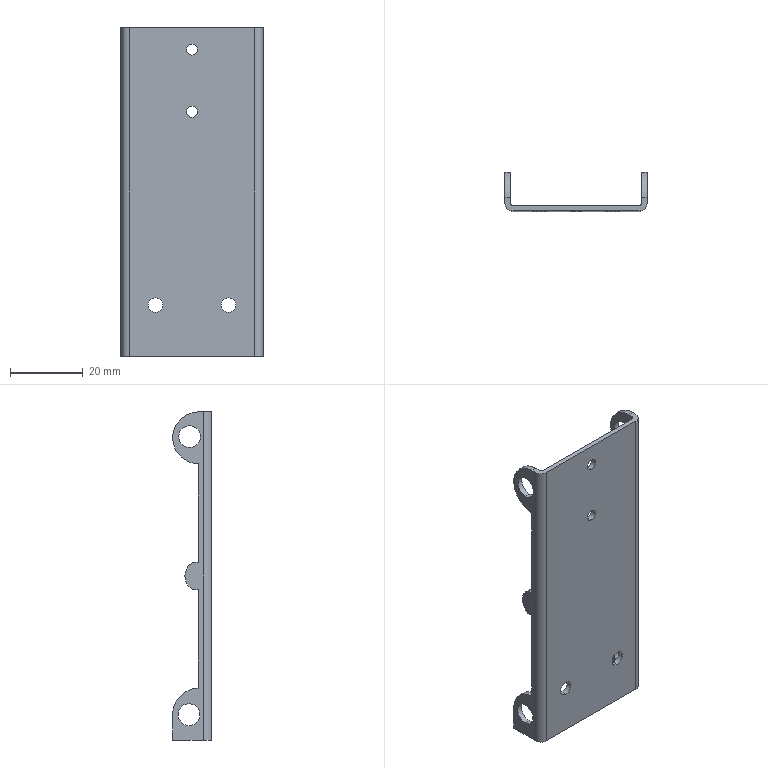Part | SolidWorks | features HoleWzd 4, Fillet 2, ICE 2, Extrusion 1 | 1 solid | 46 faces | box 39 x 10.638 x 90 mm | volume 6007 mm3 | cylinder 28 | plane 18 | commonest cylinder face diameters 6 x8 3 x4 4 x4 9.055 x4 1.473 x2 4.473 x2
STEP:
#1=CARTESIAN_POINT('',(-9.5,-1.5,-7.5));
#2=VERTEX_POINT('',#1);
#3=CARTESIAN_POINT('',(-9.5,-1.5,-4.5));
#4=VERTEX_POINT('',#3);
#5=CARTESIAN_POINT('',(-9.5,-1.5,-6.));
#6=DIRECTION('',(0.,1.,0.));
#7=DIRECTION('',(0.,0.,1.));
#8=AXIS2_PLACEMENT_3D('',#5,#6,#7);
#9=CIRCLE('',#8,1.5);
#10=EDGE_CURVE('',#2,#4,#9,.T.);
#11=ORIENTED_EDGE('',*,*,#10,.F.);
#12=CARTESIAN_POINT('',(-9.5,0.,-7.5));
#13=VERTEX_POINT('',#12);
#14=CARTESIAN_POINT('',(-9.5,0.,-7.5));
#15=DIRECTION('',(0.,1.,0.));
#16=VECTOR('',#15,1000.);
#17=LINE('',#14,#16);
#18=EDGE_CURVE('',#2,#13,#17,.T.);
#19=ORIENTED_EDGE('',*,*,#18,.T.);
#20=CARTESIAN_POINT('',(-9.5,0.,-4.5));
#21=VERTEX_POINT('',#20);
#22=CARTESIAN_POINT('',(-9.5,0.,-6.));
#23=DIRECTION('',(0.,1.,0.));
#24=DIRECTION('',(0.,0.,1.));
#25=AXIS2_PLACEMENT_3D('',#22,#23,#24);
#26=CIRCLE('',#25,1.5);
#27=EDGE_CURVE('',#13,#21,#26,.T.);
#28=ORIENTED_EDGE('',*,*,#27,.T.);
#29=CARTESIAN_POINT('',(-9.5,0.,-4.5));
#30=DIRECTION('',(0.,1.,0.));
#31=VECTOR('',#30,1000.);
#32=LINE('',#29,#31);
#33=EDGE_CURVE('',#4,#21,#32,.T.);
#34=ORIENTED_EDGE('',*,*,#33,.F.);
#35=EDGE_LOOP('',(#11,#19,#28,#34));
#36=FACE_OUTER_BOUND('',#35,.T.);
#37=CARTESIAN_POINT('',(-9.5,0.,-6.));
#38=DIRECTION('',(0.,1.,0.));
#39=DIRECTION('',(0.,0.,1.));
#40=AXIS2_PLACEMENT_3D('',#37,#38,#39);
#41=CYLINDRICAL_SURFACE('',#40,1.5);
#42=ADVANCED_FACE('',(#36),#41,.F.);
#43=CARTESIAN_POINT('',(-9.5,-1.5,-24.5));
#44=VERTEX_POINT('',#43);
#45=CARTESIAN_POINT('',(-9.5,-1.5,-21.5));
#46=VERTEX_POINT('',#45);
#47=CARTESIAN_POINT('',(-9.5,-1.5,-23.));
#48=DIRECTION('',(0.,1.,0.));
#49=DIRECTION('',(0.,0.,1.));
#50=AXIS2_PLACEMENT_3D('',#47,#48,#49);
#51=CIRCLE('',#50,1.5);
#52=EDGE_CURVE('',#44,#46,#51,.T.);
#53=ORIENTED_EDGE('',*,*,#52,.F.);
#54=CARTESIAN_POINT('',(-9.5,0.,-24.5));
#55=VERTEX_POINT('',#54);
#56=CARTESIAN_POINT('',(-9.5,0.,-24.5));
#57=DIRECTION('',(0.,1.,0.));
#58=VECTOR('',#57,1000.);
#59=LINE('',#56,#58);
#60=EDGE_CURVE('',#44,#55,#59,.T.);
#61=ORIENTED_EDGE('',*,*,#60,.T.);
#62=CARTESIAN_POINT('',(-9.5,0.,-21.5));
#63=VERTEX_POINT('',#62);
#64=CARTESIAN_POINT('',(-9.5,0.,-23.));
#65=DIRECTION('',(0.,1.,0.));
#66=DIRECTION('',(0.,0.,1.));
#67=AXIS2_PLACEMENT_3D('',#64,#65,#66);
#68=CIRCLE('',#67,1.5);
#69=EDGE_CURVE('',#55,#63,#68,.T.);
#70=ORIENTED_EDGE('',*,*,#69,.T.);
#71=CARTESIAN_POINT('',(-9.5,0.,-21.5));
#72=DIRECTION('',(0.,1.,0.));
#73=VECTOR('',#72,1000.);
#74=LINE('',#71,#73);
#75=EDGE_CURVE('',#46,#63,#74,.T.);
#76=ORIENTED_EDGE('',*,*,#75,.F.);
#77=EDGE_LOOP('',(#53,#61,#70,#76));
#78=FACE_OUTER_BOUND('',#77,.T.);
#79=CARTESIAN_POINT('',(-9.5,0.,-23.));
#80=DIRECTION('',(0.,1.,0.));
#81=DIRECTION('',(0.,0.,1.));
#82=AXIS2_PLACEMENT_3D('',#79,#80,#81);
#83=CYLINDRICAL_SURFACE('',#82,1.5);
#84=ADVANCED_FACE('',(#78),#83,.F.);
#85=CARTESIAN_POINT('',(-19.5,-1.5,-78.));
#86=VERTEX_POINT('',#85);
#87=CARTESIAN_POINT('',(-19.5,-1.5,-74.));
#88=VERTEX_POINT('',#87);
#89=CARTESIAN_POINT('',(-19.5,-1.5,-76.));
#90=DIRECTION('',(0.,1.,0.));
#91=DIRECTION('',(0.,0.,1.));
#92=AXIS2_PLACEMENT_3D('',#89,#90,#91);
#93=CIRCLE('',#92,2.);
#94=EDGE_CURVE('',#86,#88,#93,.T.);
#95=ORIENTED_EDGE('',*,*,#94,.F.);
#96=CARTESIAN_POINT('',(-19.5,0.,-78.));
#97=VERTEX_POINT('',#96);
#98=CARTESIAN_POINT('',(-19.5,0.,-78.));
#99=DIRECTION('',(0.,1.,0.));
#100=VECTOR('',#99,1000.);
#101=LINE('',#98,#100);
#102=EDGE_CURVE('',#86,#97,#101,.T.);
#103=ORIENTED_EDGE('',*,*,#102,.T.);
#104=CARTESIAN_POINT('',(-19.5,0.,-74.));
#105=VERTEX_POINT('',#104);
#106=CARTESIAN_POINT('',(-19.5,0.,-76.));
#107=DIRECTION('',(0.,1.,0.));
#108=DIRECTION('',(0.,0.,1.));
#109=AXIS2_PLACEMENT_3D('',#106,#107,#108);
#110=CIRCLE('',#109,2.);
#111=EDGE_CURVE('',#97,#105,#110,.T.);
#112=ORIENTED_EDGE('',*,*,#111,.T.);
#113=CARTESIAN_POINT('',(-19.5,0.,-74.));
#114=DIRECTION('',(0.,1.,0.));
#115=VECTOR('',#114,1000.);
#116=LINE('',#113,#115);
#117=EDGE_CURVE('',#88,#105,#116,.T.);
#118=ORIENTED_EDGE('',*,*,#117,.F.);
#119=EDGE_LOOP('',(#95,#103,#112,#118));
#120=FACE_OUTER_BOUND('',#119,.T.);
#121=CARTESIAN_POINT('',(-19.5,0.,-76.));
#122=DIRECTION('',(0.,1.,0.));
#123=DIRECTION('',(0.,0.,1.));
#124=AXIS2_PLACEMENT_3D('',#121,#122,#123);
#125=CYLINDRICAL_SURFACE('',#124,2.);
#126=ADVANCED_FACE('',(#120),#125,.F.);
#127=CARTESIAN_POINT('',(0.5,-1.5,-78.));
#128=VERTEX_POINT('',#127);
#129=CARTESIAN_POINT('',(0.5,-1.5,-74.));
#130=VERTEX_POINT('',#129);
#131=CARTESIAN_POINT('',(0.5,-1.5,-76.));
#132=DIRECTION('',(0.,1.,0.));
#133=DIRECTION('',(0.,0.,1.));
#134=AXIS2_PLACEMENT_3D('',#131,#132,#133);
#135=CIRCLE('',#134,2.);
#136=EDGE_CURVE('',#128,#130,#135,.T.);
#137=ORIENTED_EDGE('',*,*,#136,.F.);
#138=CARTESIAN_POINT('',(0.5,0.,-78.));
#139=VERTEX_POINT('',#138);
#140=CARTESIAN_POINT('',(0.5,0.,-78.));
#141=DIRECTION('',(0.,1.,0.));
#142=VECTOR('',#141,1000.);
#143=LINE('',#140,#142);
#144=EDGE_CURVE('',#128,#139,#143,.T.);
#145=ORIENTED_EDGE('',*,*,#144,.T.);
#146=CARTESIAN_POINT('',(0.5,0.,-74.));
#147=VERTEX_POINT('',#146);
#148=CARTESIAN_POINT('',(0.5,0.,-76.));
#149=DIRECTION('',(0.,1.,0.));
#150=DIRECTION('',(0.,0.,1.));
#151=AXIS2_PLACEMENT_3D('',#148,#149,#150);
#152=CIRCLE('',#151,2.);
#153=EDGE_CURVE('',#139,#147,#152,.T.);
#154=ORIENTED_EDGE('',*,*,#153,.T.);
#155=CARTESIAN_POINT('',(0.5,0.,-74.));
#156=DIRECTION('',(0.,1.,0.));
#157=VECTOR('',#156,1000.);
#158=LINE('',#155,#157);
#159=EDGE_CURVE('',#130,#147,#158,.T.);
#160=ORIENTED_EDGE('',*,*,#159,.F.);
#161=EDGE_LOOP('',(#137,#145,#154,#160));
#162=FACE_OUTER_BOUND('',#161,.T.);
#163=CARTESIAN_POINT('',(0.5,0.,-76.));
#164=DIRECTION('',(0.,1.,0.));
#165=DIRECTION('',(0.,0.,1.));
#166=AXIS2_PLACEMENT_3D('',#163,#164,#165);
#167=CYLINDRICAL_SURFACE('',#166,2.);
#168=ADVANCED_FACE('',(#162),#167,.F.);
#169=CARTESIAN_POINT('',(-29.,4.638,-80.));
#170=VERTEX_POINT('',#169);
#171=CARTESIAN_POINT('',(-29.,4.638,-86.));
#172=VERTEX_POINT('',#171);
#173=CARTESIAN_POINT('',(-29.,4.638,-83.));
#174=DIRECTION('',(1.,0.,0.));
#175=DIRECTION('',(0.,0.,-1.));
#176=AXIS2_PLACEMENT_3D('',#173,#174,#175);
#177=CIRCLE('',#176,3.);
#178=EDGE_CURVE('',#170,#172,#177,.T.);
#179=ORIENTED_EDGE('',*,*,#178,.F.);
#180=CARTESIAN_POINT('',(-27.5,4.638,-80.));
#181=VERTEX_POINT('',#180);
#182=CARTESIAN_POINT('',(-27.5,4.638,-80.));
#183=DIRECTION('',(1.,0.,0.));
#184=VECTOR('',#183,1000.);
#185=LINE('',#182,#184);
#186=EDGE_CURVE('',#170,#181,#185,.T.);
#187=ORIENTED_EDGE('',*,*,#186,.T.);
#188=CARTESIAN_POINT('',(-27.5,4.638,-86.));
#189=VERTEX_POINT('',#188);
#190=CARTESIAN_POINT('',(-27.5,4.638,-83.));
#191=DIRECTION('',(1.,0.,0.));
#192=DIRECTION('',(0.,0.,-1.));
#193=AXIS2_PLACEMENT_3D('',#190,#191,#192);
#194=CIRCLE('',#193,3.);
#195=EDGE_CURVE('',#181,#189,#194,.T.);
#196=ORIENTED_EDGE('',*,*,#195,.T.);
#197=CARTESIAN_POINT('',(-27.5,4.638,-86.));
#198=DIRECTION('',(1.,0.,0.));
#199=VECTOR('',#198,1000.);
#200=LINE('',#197,#199);
#201=EDGE_CURVE('',#172,#189,#200,.T.);
#202=ORIENTED_EDGE('',*,*,#201,.F.);
#203=EDGE_LOOP('',(#179,#187,#196,#202));
#204=FACE_OUTER_BOUND('',#203,.T.);
#205=CARTESIAN_POINT('',(-27.5,4.638,-83.));
#206=DIRECTION('',(1.,0.,0.));
#207=DIRECTION('',(0.,0.,-1.));
#208=AXIS2_PLACEMENT_3D('',#205,#206,#207);
#209=CYLINDRICAL_SURFACE('',#208,3.);
#210=ADVANCED_FACE('',(#204),#209,.F.);
#211=CARTESIAN_POINT('',(-29.,4.482,-3.846));
#212=VERTEX_POINT('',#211);
#213=CARTESIAN_POINT('',(-29.,4.482,-9.846));
#214=VERTEX_POINT('',#213);
#215=CARTESIAN_POINT('',(-29.,4.482,-6.846));
#216=DIRECTION('',(1.,0.,0.));
#217=DIRECTION('',(0.,0.,-1.));
#218=AXIS2_PLACEMENT_3D('',#215,#216,#217);
#219=CIRCLE('',#218,3.);
#220=EDGE_CURVE('',#212,#214,#219,.T.);
#221=ORIENTED_EDGE('',*,*,#220,.F.);
#222=CARTESIAN_POINT('',(-27.5,4.482,-3.846));
#223=VERTEX_POINT('',#222);
#224=CARTESIAN_POINT('',(-27.5,4.482,-3.846));
#225=DIRECTION('',(1.,0.,0.));
#226=VECTOR('',#225,1000.);
#227=LINE('',#224,#226);
#228=EDGE_CURVE('',#212,#223,#227,.T.);
#229=ORIENTED_EDGE('',*,*,#228,.T.);
#230=CARTESIAN_POINT('',(-27.5,4.482,-9.846));
#231=VERTEX_POINT('',#230);
#232=CARTESIAN_POINT('',(-27.5,4.482,-6.846));
#233=DIRECTION('',(1.,0.,0.));
#234=DIRECTION('',(0.,0.,-1.));
#235=AXIS2_PLACEMENT_3D('',#232,#233,#234);
#236=CIRCLE('',#235,3.);
#237=EDGE_CURVE('',#223,#231,#236,.T.);
#238=ORIENTED_EDGE('',*,*,#237,.T.);
#239=CARTESIAN_POINT('',(-27.5,4.482,-9.846));
#240=DIRECTION('',(1.,0.,0.));
#241=VECTOR('',#240,1000.);
#242=LINE('',#239,#241);
#243=EDGE_CURVE('',#214,#231,#242,.T.);
#244=ORIENTED_EDGE('',*,*,#243,.F.);
#245=EDGE_LOOP('',(#221,#229,#238,#244));
#246=FACE_OUTER_BOUND('',#245,.T.);
#247=CARTESIAN_POINT('',(-27.5,4.482,-6.846));
#248=DIRECTION('',(1.,0.,0.));
#249=DIRECTION('',(0.,0.,-1.));
#250=AXIS2_PLACEMENT_3D('',#247,#248,#249);
#251=CYLINDRICAL_SURFACE('',#250,3.);
#252=ADVANCED_FACE('',(#246),#251,.F.);
#253=CARTESIAN_POINT('',(10.,4.482,-9.846));
#254=VERTEX_POINT('',#253);
#255=CARTESIAN_POINT('',(10.,4.482,-3.846));
#256=VERTEX_POINT('',#255);
#257=CARTESIAN_POINT('',(10.,4.482,-6.846));
#258=DIRECTION('',(-1.,0.,0.));
#259=DIRECTION('',(0.,0.,1.));
#260=AXIS2_PLACEMENT_3D('',#257,#258,#259);
#261=CIRCLE('',#260,3.);
#262=EDGE_CURVE('',#254,#256,#261,.T.);
#263=ORIENTED_EDGE('',*,*,#262,.F.);
#264=CARTESIAN_POINT('',(8.5,4.482,-9.846));
#265=VERTEX_POINT('',#264);
#266=CARTESIAN_POINT('',(8.5,4.482,-9.846));
#267=DIRECTION('',(-1.,0.,0.));
#268=VECTOR('',#267,1000.);
#269=LINE('',#266,#268);
#270=EDGE_CURVE('',#254,#265,#269,.T.);
#271=ORIENTED_EDGE('',*,*,#270,.T.);
#272=CARTESIAN_POINT('',(8.5,4.482,-3.846));
#273=VERTEX_POINT('',#272);
#274=CARTESIAN_POINT('',(8.5,4.482,-6.846));
#275=DIRECTION('',(-1.,0.,0.));
#276=DIRECTION('',(0.,0.,1.));
#277=AXIS2_PLACEMENT_3D('',#274,#275,#276);
#278=CIRCLE('',#277,3.);
#279=EDGE_CURVE('',#265,#273,#278,.T.);
#280=ORIENTED_EDGE('',*,*,#279,.T.);
#281=CARTESIAN_POINT('',(8.5,4.482,-3.846));
#282=DIRECTION('',(-1.,0.,0.));
#283=VECTOR('',#282,1000.);
#284=LINE('',#281,#283);
#285=EDGE_CURVE('',#256,#273,#284,.T.);
#286=ORIENTED_EDGE('',*,*,#285,.F.);
#287=EDGE_LOOP('',(#263,#271,#280,#286));
#288=FACE_OUTER_BOUND('',#287,.T.);
#289=CARTESIAN_POINT('',(8.5,4.482,-6.846));
#290=DIRECTION('',(-1.,0.,0.));
#291=DIRECTION('',(0.,0.,1.));
#292=AXIS2_PLACEMENT_3D('',#289,#290,#291);
#293=CYLINDRICAL_SURFACE('',#292,3.);
#294=ADVANCED_FACE('',(#288),#293,.F.);
#295=CARTESIAN_POINT('',(10.,4.638,-86.));
#296=VERTEX_POINT('',#295);
#297=CARTESIAN_POINT('',(10.,4.638,-80.));
#298=VERTEX_POINT('',#297);
#299=CARTESIAN_POINT('',(10.,4.638,-83.));
#300=DIRECTION('',(-1.,0.,0.));
#301=DIRECTION('',(0.,0.,1.));
#302=AXIS2_PLACEMENT_3D('',#299,#300,#301);
#303=CIRCLE('',#302,3.);
#304=EDGE_CURVE('',#296,#298,#303,.T.);
#305=ORIENTED_EDGE('',*,*,#304,.F.);
#306=CARTESIAN_POINT('',(8.5,4.638,-86.));
#307=VERTEX_POINT('',#306);
#308=CARTESIAN_POINT('',(8.5,4.638,-86.));
#309=DIRECTION('',(-1.,0.,0.));
#310=VECTOR('',#309,1000.);
#311=LINE('',#308,#310);
#312=EDGE_CURVE('',#296,#307,#311,.T.);
#313=ORIENTED_EDGE('',*,*,#312,.T.);
#314=CARTESIAN_POINT('',(8.5,4.638,-80.));
#315=VERTEX_POINT('',#314);
#316=CARTESIAN_POINT('',(8.5,4.638,-83.));
#317=DIRECTION('',(-1.,0.,0.));
#318=DIRECTION('',(0.,0.,1.));
#319=AXIS2_PLACEMENT_3D('',#316,#317,#318);
#320=CIRCLE('',#319,3.);
#321=EDGE_CURVE('',#307,#315,#320,.T.);
#322=ORIENTED_EDGE('',*,*,#321,.T.);
#323=CARTESIAN_POINT('',(8.5,4.638,-80.));
#324=DIRECTION('',(-1.,0.,0.));
#325=VECTOR('',#324,1000.);
#326=LINE('',#323,#325);
#327=EDGE_CURVE('',#298,#315,#326,.T.);
#328=ORIENTED_EDGE('',*,*,#327,.F.);
#329=EDGE_LOOP('',(#305,#313,#322,#328));
#330=FACE_OUTER_BOUND('',#329,.T.);
#331=CARTESIAN_POINT('',(8.5,4.638,-83.));
#332=DIRECTION('',(-1.,0.,0.));
#333=DIRECTION('',(0.,0.,1.));
#334=AXIS2_PLACEMENT_3D('',#331,#332,#333);
#335=CYLINDRICAL_SURFACE('',#334,3.);
#336=ADVANCED_FACE('',(#330),#335,.F.);
#337=CARTESIAN_POINT('',(-27.5,4.638,-83.));
#338=DIRECTION('',(1.,0.,0.));
#339=DIRECTION('',(0.,0.,-1.));
#340=AXIS2_PLACEMENT_3D('',#337,#338,#339);
#341=CIRCLE('',#340,3.);
#342=EDGE_CURVE('',#189,#181,#341,.T.);
#343=ORIENTED_EDGE('',*,*,#342,.F.);
#344=ORIENTED_EDGE('',*,*,#195,.F.);
#345=EDGE_LOOP('',(#343,#344));
#346=FACE_BOUND('',#345,.T.);
#347=CARTESIAN_POINT('',(-27.5,0.7366,0.));
#348=VERTEX_POINT('',#347);
#349=CARTESIAN_POINT('',(-27.5,2.129,0.));
#350=VERTEX_POINT('',#349);
#351=CARTESIAN_POINT('',(-27.5,-1.5,0.));
#352=DIRECTION('',(0.,1.,0.));
#353=VECTOR('',#352,1000.);
#354=LINE('',#351,#353);
#355=EDGE_CURVE('',#348,#350,#354,.T.);
#356=ORIENTED_EDGE('',*,*,#355,.F.);
#357=CARTESIAN_POINT('',(-27.5,0.7366,-90.));
#358=VERTEX_POINT('',#357);
#359=CARTESIAN_POINT('',(-27.5,0.7366,-90.));
#360=DIRECTION('',(0.,0.,-1.));
#361=VECTOR('',#360,1000.);
#362=LINE('',#359,#361);
#363=EDGE_CURVE('',#348,#358,#362,.T.);
#364=ORIENTED_EDGE('',*,*,#363,.T.);
#365=CARTESIAN_POINT('',(-27.5,9.138,-90.));
#366=VERTEX_POINT('',#365);
#367=CARTESIAN_POINT('',(-27.5,9.138,-90.));
#368=DIRECTION('',(0.,-1.,0.));
#369=VECTOR('',#368,1000.);
#370=LINE('',#367,#369);
#371=EDGE_CURVE('',#366,#358,#370,.T.);
#372=ORIENTED_EDGE('',*,*,#371,.F.);
#373=CARTESIAN_POINT('',(-27.5,9.138,-83.));
#374=VERTEX_POINT('',#373);
#375=CARTESIAN_POINT('',(-27.5,9.138,-83.));
#376=DIRECTION('',(0.,0.,-1.));
#377=VECTOR('',#376,1000.);
#378=LINE('',#375,#377);
#379=EDGE_CURVE('',#374,#366,#378,.T.);
#380=ORIENTED_EDGE('',*,*,#379,.F.);
#381=CARTESIAN_POINT('',(-27.5,2.138,-75.731));
#382=VERTEX_POINT('',#381);
#383=CARTESIAN_POINT('',(-27.5,1.864,-83.));
#384=DIRECTION('',(-1.,0.,0.));
#385=DIRECTION('',(0.,-1.,0.));
#386=AXIS2_PLACEMENT_3D('',#383,#384,#385);
#387=CIRCLE('',#386,7.274);
#388=EDGE_CURVE('',#382,#374,#387,.T.);
#389=ORIENTED_EDGE('',*,*,#388,.F.);
#390=CARTESIAN_POINT('',(-27.5,2.138,-48.731));
#391=VERTEX_POINT('',#390);
#392=CARTESIAN_POINT('',(-27.5,2.138,-48.731));
#393=DIRECTION('',(0.,0.,-1.));
#394=VECTOR('',#393,1000.);
#395=LINE('',#392,#394);
#396=EDGE_CURVE('',#391,#382,#395,.T.);
#397=ORIENTED_EDGE('',*,*,#396,.F.);
#398=CARTESIAN_POINT('',(-27.5,3.638,-48.731));
#399=VERTEX_POINT('',#398);
#400=CARTESIAN_POINT('',(-27.5,3.638,-48.731));
#401=DIRECTION('',(0.,-1.,0.));
#402=VECTOR('',#401,1000.);
#403=LINE('',#400,#402);
#404=EDGE_CURVE('',#399,#391,#403,.T.);
#405=ORIENTED_EDGE('',*,*,#404,.F.);
#406=CARTESIAN_POINT('',(-27.5,5.778,-44.873));
#407=VERTEX_POINT('',#406);
#408=CARTESIAN_POINT('',(-27.5,1.251,-44.884));
#409=DIRECTION('',(-1.,0.,0.));
#410=DIRECTION('',(0.,-1.,0.));
#411=AXIS2_PLACEMENT_3D('',#408,#409,#410);
#412=CIRCLE('',#411,4.528);
#413=EDGE_CURVE('',#407,#399,#412,.T.);
#414=ORIENTED_EDGE('',*,*,#413,.F.);
#415=CARTESIAN_POINT('',(-27.5,3.629,-41.262));
#416=VERTEX_POINT('',#415);
#417=CARTESIAN_POINT('',(-27.5,1.257,-45.119));
#418=DIRECTION('',(-1.,0.,0.));
#419=DIRECTION('',(0.,-1.,0.));
#420=AXIS2_PLACEMENT_3D('',#417,#418,#419);
#421=CIRCLE('',#420,4.528);
#422=EDGE_CURVE('',#416,#407,#421,.T.);
#423=ORIENTED_EDGE('',*,*,#422,.F.);
#424=CARTESIAN_POINT('',(-27.5,2.129,-41.262));
#425=VERTEX_POINT('',#424);
#426=CARTESIAN_POINT('',(-27.5,2.129,-41.262));
#427=DIRECTION('',(0.,1.,0.));
#428=VECTOR('',#427,1000.);
#429=LINE('',#426,#428);
#430=EDGE_CURVE('',#425,#416,#429,.T.);
#431=ORIENTED_EDGE('',*,*,#430,.F.);
#432=CARTESIAN_POINT('',(-27.5,2.129,-14.262));
#433=VERTEX_POINT('',#432);
#434=CARTESIAN_POINT('',(-27.5,2.129,-14.262));
#435=DIRECTION('',(0.,0.,-1.));
#436=VECTOR('',#435,1000.);
#437=LINE('',#434,#436);
#438=EDGE_CURVE('',#433,#425,#437,.T.);
#439=ORIENTED_EDGE('',*,*,#438,.F.);
#440=CARTESIAN_POINT('',(-27.5,1.998,-7.131));
#441=DIRECTION('',(-1.,0.,0.));
#442=DIRECTION('',(0.,-1.,0.));
#443=AXIS2_PLACEMENT_3D('',#440,#441,#442);
#444=CIRCLE('',#443,7.132);
#445=EDGE_CURVE('',#350,#433,#444,.T.);
#446=ORIENTED_EDGE('',*,*,#445,.F.);
#447=EDGE_LOOP('',(#356,#364,#372,#380,#389,#397,#405,#414,#423,#431,#439,#446));
#448=FACE_OUTER_BOUND('',#447,.T.);
#449=CARTESIAN_POINT('',(-27.5,4.482,-6.846));
#450=DIRECTION('',(1.,0.,0.));
#451=DIRECTION('',(0.,0.,-1.));
#452=AXIS2_PLACEMENT_3D('',#449,#450,#451);
#453=CIRCLE('',#452,3.);
#454=EDGE_CURVE('',#231,#223,#453,.T.);
#455=ORIENTED_EDGE('',*,*,#454,.F.);
#456=ORIENTED_EDGE('',*,*,#237,.F.);
#457=EDGE_LOOP('',(#455,#456));
#458=FACE_BOUND('',#457,.T.);
#459=CARTESIAN_POINT('',(-27.5,1.998,-7.131));
#460=DIRECTION('',(-1.,0.,0.));
#461=DIRECTION('',(0.,-1.,0.));
#462=AXIS2_PLACEMENT_3D('',#459,#460,#461);
#463=PLANE('',#462);
#464=ADVANCED_FACE('',(#346,#448,#458),#463,.F.);
#465=CARTESIAN_POINT('',(-29.,9.138,-83.));
#466=VERTEX_POINT('',#465);
#467=CARTESIAN_POINT('',(-29.,9.138,-90.));
#468=VERTEX_POINT('',#467);
#469=CARTESIAN_POINT('',(-29.,9.138,-83.));
#470=DIRECTION('',(0.,0.,-1.));
#471=VECTOR('',#470,1000.);
#472=LINE('',#469,#471);
#473=EDGE_CURVE('',#466,#468,#472,.T.);
#474=ORIENTED_EDGE('',*,*,#473,.F.);
#475=CARTESIAN_POINT('',(-27.5,9.138,-83.));
#476=DIRECTION('',(-1.,0.,0.));
#477=VECTOR('',#476,1000.);
#478=LINE('',#475,#477);
#479=EDGE_CURVE('',#374,#466,#478,.T.);
#480=ORIENTED_EDGE('',*,*,#479,.F.);
#481=ORIENTED_EDGE('',*,*,#379,.T.);
#482=CARTESIAN_POINT('',(-27.5,9.138,-90.));
#483=DIRECTION('',(-1.,0.,0.));
#484=VECTOR('',#483,1000.);
#485=LINE('',#482,#484);
#486=EDGE_CURVE('',#366,#468,#485,.T.);
#487=ORIENTED_EDGE('',*,*,#486,.T.);
#488=EDGE_LOOP('',(#474,#480,#481,#487));
#489=FACE_OUTER_BOUND('',#488,.T.);
#490=CARTESIAN_POINT('',(-27.5,9.138,-83.));
#491=DIRECTION('',(0.,1.,0.));
#492=DIRECTION('',(-1.,0.,0.));
#493=AXIS2_PLACEMENT_3D('',#490,#491,#492);
#494=PLANE('',#493);
#495=ADVANCED_FACE('',(#489),#494,.T.);
#496=CARTESIAN_POINT('',(-29.,2.138,-75.731));
#497=VERTEX_POINT('',#496);
#498=CARTESIAN_POINT('',(-29.,1.864,-83.));
#499=DIRECTION('',(-1.,0.,0.));
#500=DIRECTION('',(0.,-1.,0.));
#501=AXIS2_PLACEMENT_3D('',#498,#499,#500);
#502=CIRCLE('',#501,7.274);
#503=EDGE_CURVE('',#497,#466,#502,.T.);
#504=ORIENTED_EDGE('',*,*,#503,.F.);
#505=CARTESIAN_POINT('',(-27.5,2.138,-75.731));
#506=DIRECTION('',(-1.,0.,0.));
#507=VECTOR('',#506,1000.);
#508=LINE('',#505,#507);
#509=EDGE_CURVE('',#382,#497,#508,.T.);
#510=ORIENTED_EDGE('',*,*,#509,.F.);
#511=ORIENTED_EDGE('',*,*,#388,.T.);
#512=ORIENTED_EDGE('',*,*,#479,.T.);
#513=EDGE_LOOP('',(#504,#510,#511,#512));
#514=FACE_OUTER_BOUND('',#513,.T.);
#515=CARTESIAN_POINT('',(-27.5,1.864,-83.));
#516=DIRECTION('',(-1.,0.,0.));
#517=DIRECTION('',(0.,-1.,0.));
#518=AXIS2_PLACEMENT_3D('',#515,#516,#517);
#519=CYLINDRICAL_SURFACE('',#518,7.274);
#520=ADVANCED_FACE('',(#514),#519,.T.);
#521=CARTESIAN_POINT('',(-29.,2.138,-48.731));
#522=VERTEX_POINT('',#521);
#523=CARTESIAN_POINT('',(-29.,2.138,-48.731));
#524=DIRECTION('',(0.,0.,-1.));
#525=VECTOR('',#524,1000.);
#526=LINE('',#523,#525);
#527=EDGE_CURVE('',#522,#497,#526,.T.);
#528=ORIENTED_EDGE('',*,*,#527,.F.);
#529=CARTESIAN_POINT('',(-27.5,2.138,-48.731));
#530=DIRECTION('',(-1.,0.,0.));
#531=VECTOR('',#530,1000.);
#532=LINE('',#529,#531);
#533=EDGE_CURVE('',#391,#522,#532,.T.);
#534=ORIENTED_EDGE('',*,*,#533,.F.);
#535=ORIENTED_EDGE('',*,*,#396,.T.);
#536=ORIENTED_EDGE('',*,*,#509,.T.);
#537=EDGE_LOOP('',(#528,#534,#535,#536));
#538=FACE_OUTER_BOUND('',#537,.T.);
#539=CARTESIAN_POINT('',(-27.5,2.138,-48.731));
#540=DIRECTION('',(0.,1.,0.));
#541=DIRECTION('',(-1.,0.,0.));
#542=AXIS2_PLACEMENT_3D('',#539,#540,#541);
#543=PLANE('',#542);
#544=ADVANCED_FACE('',(#538),#543,.T.);
#545=CARTESIAN_POINT('',(-29.,3.638,-48.731));
#546=VERTEX_POINT('',#545);
#547=CARTESIAN_POINT('',(-29.,3.638,-48.731));
#548=DIRECTION('',(0.,-1.,0.));
#549=VECTOR('',#548,1000.);
#550=LINE('',#547,#549);
#551=EDGE_CURVE('',#546,#522,#550,.T.);
#552=ORIENTED_EDGE('',*,*,#551,.F.);
#553=CARTESIAN_POINT('',(-27.5,3.638,-48.731));
#554=DIRECTION('',(-1.,0.,0.));
#555=VECTOR('',#554,1000.);
#556=LINE('',#553,#555);
#557=EDGE_CURVE('',#399,#546,#556,.T.);
#558=ORIENTED_EDGE('',*,*,#557,.F.);
#559=ORIENTED_EDGE('',*,*,#404,.T.);
#560=ORIENTED_EDGE('',*,*,#533,.T.);
#561=EDGE_LOOP('',(#552,#558,#559,#560));
#562=FACE_OUTER_BOUND('',#561,.T.);
#563=CARTESIAN_POINT('',(-27.5,3.638,-48.731));
#564=DIRECTION('',(0.,0.,-1.));
#565=DIRECTION('',(-1.,0.,0.));
#566=AXIS2_PLACEMENT_3D('',#563,#564,#565);
#567=PLANE('',#566);
#568=ADVANCED_FACE('',(#562),#567,.T.);
#569=CARTESIAN_POINT('',(-29.,5.778,-44.873));
#570=VERTEX_POINT('',#569);
#571=CARTESIAN_POINT('',(-29.,1.251,-44.884));
#572=DIRECTION('',(-1.,0.,0.));
#573=DIRECTION('',(0.,-1.,0.));
#574=AXIS2_PLACEMENT_3D('',#571,#572,#573);
#575=CIRCLE('',#574,4.528);
#576=EDGE_CURVE('',#570,#546,#575,.T.);
#577=ORIENTED_EDGE('',*,*,#576,.F.);
#578=CARTESIAN_POINT('',(-27.5,5.778,-44.873));
#579=DIRECTION('',(-1.,0.,0.));
#580=VECTOR('',#579,1000.);
#581=LINE('',#578,#580);
#582=EDGE_CURVE('',#407,#570,#581,.T.);
#583=ORIENTED_EDGE('',*,*,#582,.F.);
#584=ORIENTED_EDGE('',*,*,#413,.T.);
#585=ORIENTED_EDGE('',*,*,#557,.T.);
#586=EDGE_LOOP('',(#577,#583,#584,#585));
#587=FACE_OUTER_BOUND('',#586,.T.);
#588=CARTESIAN_POINT('',(-27.5,1.251,-44.884));
#589=DIRECTION('',(-1.,0.,0.));
#590=DIRECTION('',(0.,-1.,0.));
#591=AXIS2_PLACEMENT_3D('',#588,#589,#590);
#592=CYLINDRICAL_SURFACE('',#591,4.528);
#593=ADVANCED_FACE('',(#587),#592,.T.);
#594=CARTESIAN_POINT('',(-29.,3.629,-41.262));
#595=VERTEX_POINT('',#594);
#596=CARTESIAN_POINT('',(-29.,1.257,-45.119));
#597=DIRECTION('',(-1.,0.,0.));
#598=DIRECTION('',(0.,-1.,0.));
#599=AXIS2_PLACEMENT_3D('',#596,#597,#598);
#600=CIRCLE('',#599,4.528);
#601=EDGE_CURVE('',#595,#570,#600,.T.);
#602=ORIENTED_EDGE('',*,*,#601,.F.);
#603=CARTESIAN_POINT('',(-27.5,3.629,-41.262));
#604=DIRECTION('',(-1.,0.,0.));
#605=VECTOR('',#604,1000.);
#606=LINE('',#603,#605);
#607=EDGE_CURVE('',#416,#595,#606,.T.);
#608=ORIENTED_EDGE('',*,*,#607,.F.);
#609=ORIENTED_EDGE('',*,*,#422,.T.);
#610=ORIENTED_EDGE('',*,*,#582,.T.);
#611=EDGE_LOOP('',(#602,#608,#609,#610));
#612=FACE_OUTER_BOUND('',#611,.T.);
#613=CARTESIAN_POINT('',(-27.5,1.257,-45.119));
#614=DIRECTION('',(-1.,0.,0.));
#615=DIRECTION('',(0.,-1.,0.));
#616=AXIS2_PLACEMENT_3D('',#613,#614,#615);
#617=CYLINDRICAL_SURFACE('',#616,4.528);
#618=ADVANCED_FACE('',(#612),#617,.T.);
#619=CARTESIAN_POINT('',(-29.,2.129,-41.262));
#620=VERTEX_POINT('',#619);
#621=CARTESIAN_POINT('',(-29.,2.129,-41.262));
#622=DIRECTION('',(0.,1.,0.));
#623=VECTOR('',#622,1000.);
#624=LINE('',#621,#623);
#625=EDGE_CURVE('',#620,#595,#624,.T.);
#626=ORIENTED_EDGE('',*,*,#625,.F.);
#627=CARTESIAN_POINT('',(-27.5,2.129,-41.262));
#628=DIRECTION('',(-1.,0.,0.));
#629=VECTOR('',#628,1000.);
#630=LINE('',#627,#629);
#631=EDGE_CURVE('',#425,#620,#630,.T.);
#632=ORIENTED_EDGE('',*,*,#631,.F.);
#633=ORIENTED_EDGE('',*,*,#430,.T.);
#634=ORIENTED_EDGE('',*,*,#607,.T.);
#635=EDGE_LOOP('',(#626,#632,#633,#634));
#636=FACE_OUTER_BOUND('',#635,.T.);
#637=CARTESIAN_POINT('',(-27.5,2.129,-41.262));
#638=DIRECTION('',(0.,0.,1.));
#639=DIRECTION('',(1.,0.,0.));
#640=AXIS2_PLACEMENT_3D('',#637,#638,#639);
#641=PLANE('',#640);
#642=ADVANCED_FACE('',(#636),#641,.T.);
#643=CARTESIAN_POINT('',(-29.,2.129,-14.262));
#644=VERTEX_POINT('',#643);
#645=CARTESIAN_POINT('',(-29.,2.129,-14.262));
#646=DIRECTION('',(0.,0.,-1.));
#647=VECTOR('',#646,1000.);
#648=LINE('',#645,#647);
#649=EDGE_CURVE('',#644,#620,#648,.T.);
#650=ORIENTED_EDGE('',*,*,#649,.F.);
#651=CARTESIAN_POINT('',(-27.5,2.129,-14.262));
#652=DIRECTION('',(-1.,0.,0.));
#653=VECTOR('',#652,1000.);
#654=LINE('',#651,#653);
#655=EDGE_CURVE('',#433,#644,#654,.T.);
#656=ORIENTED_EDGE('',*,*,#655,.F.);
#657=ORIENTED_EDGE('',*,*,#438,.T.);
#658=ORIENTED_EDGE('',*,*,#631,.T.);
#659=EDGE_LOOP('',(#650,#656,#657,#658));
#660=FACE_OUTER_BOUND('',#659,.T.);
#661=CARTESIAN_POINT('',(-27.5,2.129,-14.262));
#662=DIRECTION('',(0.,1.,0.));
#663=DIRECTION('',(-1.,0.,0.));
#664=AXIS2_PLACEMENT_3D('',#661,#662,#663);
#665=PLANE('',#664);
#666=ADVANCED_FACE('',(#660),#665,.T.);
#667=CARTESIAN_POINT('',(-29.,2.129,0.));
#668=VERTEX_POINT('',#667);
#669=CARTESIAN_POINT('',(-29.,1.998,-7.131));
#670=DIRECTION('',(-1.,0.,0.));
#671=DIRECTION('',(0.,-1.,0.));
#672=AXIS2_PLACEMENT_3D('',#669,#670,#671);
#673=CIRCLE('',#672,7.132);
#674=EDGE_CURVE('',#668,#644,#673,.T.);
#675=ORIENTED_EDGE('',*,*,#674,.F.);
#676=CARTESIAN_POINT('',(-27.5,2.129,0.));
#677=DIRECTION('',(-1.,0.,0.));
#678=VECTOR('',#677,1000.);
#679=LINE('',#676,#678);
#680=EDGE_CURVE('',#350,#668,#679,.T.);
#681=ORIENTED_EDGE('',*,*,#680,.F.);
#682=ORIENTED_EDGE('',*,*,#445,.T.);
#683=ORIENTED_EDGE('',*,*,#655,.T.);
#684=EDGE_LOOP('',(#675,#681,#682,#683));
#685=FACE_OUTER_BOUND('',#684,.T.);
#686=CARTESIAN_POINT('',(-27.5,1.998,-7.131));
#687=DIRECTION('',(-1.,0.,0.));
#688=DIRECTION('',(0.,-1.,0.));
#689=AXIS2_PLACEMENT_3D('',#686,#687,#688);
#690=CYLINDRICAL_SURFACE('',#689,7.132);
#691=ADVANCED_FACE('',(#685),#690,.T.);
#692=CARTESIAN_POINT('',(-29.,0.7366,0.));
#693=VERTEX_POINT('',#692);
#694=CARTESIAN_POINT('',(-29.,-1.5,0.));
#695=DIRECTION('',(0.,1.,0.));
#696=VECTOR('',#695,1000.);
#697=LINE('',#694,#696);
#698=EDGE_CURVE('',#693,#668,#697,.T.);
#699=ORIENTED_EDGE('',*,*,#698,.F.);
#700=CARTESIAN_POINT('',(-26.763,-1.5,0.));
#701=VERTEX_POINT('',#700);
#702=CARTESIAN_POINT('',(-26.763,0.7366,0.));
#703=DIRECTION('',(0.,0.,1.));
#704=DIRECTION('',(0.,-1.,0.));
#705=AXIS2_PLACEMENT_3D('',#702,#703,#704);
#706=CIRCLE('',#705,2.237);
#707=EDGE_CURVE('',#693,#701,#706,.T.);
#708=ORIENTED_EDGE('',*,*,#707,.T.);
#709=CARTESIAN_POINT('',(7.763,-1.5,0.));
#710=VERTEX_POINT('',#709);
#711=CARTESIAN_POINT('',(-27.5,-1.5,0.));
#712=DIRECTION('',(-1.,0.,0.));
#713=VECTOR('',#712,1000.);
#714=LINE('',#711,#713);
#715=EDGE_CURVE('',#710,#701,#714,.T.);
#716=ORIENTED_EDGE('',*,*,#715,.F.);
#717=CARTESIAN_POINT('',(10.,0.7366,0.));
#718=VERTEX_POINT('',#717);
#719=CARTESIAN_POINT('',(7.763,0.7366,0.));
#720=DIRECTION('',(0.,0.,1.));
#721=DIRECTION('',(0.,-1.,0.));
#722=AXIS2_PLACEMENT_3D('',#719,#720,#721);
#723=CIRCLE('',#722,2.237);
#724=EDGE_CURVE('',#710,#718,#723,.T.);
#725=ORIENTED_EDGE('',*,*,#724,.T.);
#726=CARTESIAN_POINT('',(10.,2.129,0.));
#727=VERTEX_POINT('',#726);
#728=CARTESIAN_POINT('',(10.,-1.5,0.));
#729=DIRECTION('',(0.,-1.,0.));
#730=VECTOR('',#729,1000.);
#731=LINE('',#728,#730);
#732=EDGE_CURVE('',#727,#718,#731,.T.);
#733=ORIENTED_EDGE('',*,*,#732,.F.);
#734=CARTESIAN_POINT('',(8.5,2.129,0.));
#735=VERTEX_POINT('',#734);
#736=CARTESIAN_POINT('',(10.,2.129,0.));
#737=DIRECTION('',(-1.,0.,0.));
#738=VECTOR('',#737,1000.);
#739=LINE('',#736,#738);
#740=EDGE_CURVE('',#727,#735,#739,.T.);
#741=ORIENTED_EDGE('',*,*,#740,.T.);
#742=CARTESIAN_POINT('',(8.5,0.7366,0.));
#743=VERTEX_POINT('',#742);
#744=CARTESIAN_POINT('',(8.5,-1.5,0.));
#745=DIRECTION('',(0.,-1.,0.));
#746=VECTOR('',#745,1000.);
#747=LINE('',#744,#746);
#748=EDGE_CURVE('',#735,#743,#747,.T.);
#749=ORIENTED_EDGE('',*,*,#748,.T.);
#750=CARTESIAN_POINT('',(7.763,0.,0.));
#751=VERTEX_POINT('',#750);
#752=CARTESIAN_POINT('',(7.763,0.7366,0.));
#753=DIRECTION('',(0.,0.,-1.));
#754=DIRECTION('',(0.,-1.,0.));
#755=AXIS2_PLACEMENT_3D('',#752,#753,#754);
#756=CIRCLE('',#755,0.7366);
#757=EDGE_CURVE('',#743,#751,#756,.T.);
#758=ORIENTED_EDGE('',*,*,#757,.T.);
#759=CARTESIAN_POINT('',(-26.763,0.,0.));
#760=VERTEX_POINT('',#759);
#761=CARTESIAN_POINT('',(8.5,0.,0.));
#762=DIRECTION('',(-1.,0.,0.));
#763=VECTOR('',#762,1000.);
#764=LINE('',#761,#763);
#765=EDGE_CURVE('',#751,#760,#764,.T.);
#766=ORIENTED_EDGE('',*,*,#765,.T.);
#767=CARTESIAN_POINT('',(-26.763,0.7366,0.));
#768=DIRECTION('',(0.,0.,-1.));
#769=DIRECTION('',(0.,-1.,0.));
#770=AXIS2_PLACEMENT_3D('',#767,#768,#769);
#771=CIRCLE('',#770,0.7366);
#772=EDGE_CURVE('',#760,#348,#771,.T.);
#773=ORIENTED_EDGE('',*,*,#772,.T.);
#774=ORIENTED_EDGE('',*,*,#355,.T.);
#775=ORIENTED_EDGE('',*,*,#680,.T.);
#776=EDGE_LOOP('',(#699,#708,#716,#725,#733,#741,#749,#758,#766,#773,#774,#775));
#777=FACE_OUTER_BOUND('',#776,.T.);
#778=CARTESIAN_POINT('',(-27.5,-1.5,0.));
#779=DIRECTION('',(0.,0.,1.));
#780=DIRECTION('',(0.,-1.,0.));
#781=AXIS2_PLACEMENT_3D('',#778,#779,#780);
#782=PLANE('',#781);
#783=ADVANCED_FACE('',(#777),#782,.T.);
#784=CARTESIAN_POINT('',(-9.5,-1.5,-6.));
#785=DIRECTION('',(0.,1.,0.));
#786=DIRECTION('',(0.,0.,1.));
#787=AXIS2_PLACEMENT_3D('',#784,#785,#786);
#788=CIRCLE('',#787,1.5);
#789=EDGE_CURVE('',#4,#2,#788,.T.);
#790=ORIENTED_EDGE('',*,*,#789,.T.);
#791=ORIENTED_EDGE('',*,*,#10,.T.);
#792=EDGE_LOOP('',(#790,#791));
#793=FACE_BOUND('',#792,.T.);
#794=CARTESIAN_POINT('',(-9.5,-1.5,-23.));
#795=DIRECTION('',(0.,1.,0.));
#796=DIRECTION('',(0.,0.,1.));
#797=AXIS2_PLACEMENT_3D('',#794,#795,#796);
#798=CIRCLE('',#797,1.5);
#799=EDGE_CURVE('',#46,#44,#798,.T.);
#800=ORIENTED_EDGE('',*,*,#799,.T.);
#801=ORIENTED_EDGE('',*,*,#52,.T.);
#802=EDGE_LOOP('',(#800,#801));
#803=FACE_BOUND('',#802,.T.);
#804=CARTESIAN_POINT('',(-19.5,-1.5,-76.));
#805=DIRECTION('',(0.,1.,0.));
#806=DIRECTION('',(0.,0.,1.));
#807=AXIS2_PLACEMENT_3D('',#804,#805,#806);
#808=CIRCLE('',#807,2.);
#809=EDGE_CURVE('',#88,#86,#808,.T.);
#810=ORIENTED_EDGE('',*,*,#809,.T.);
#811=ORIENTED_EDGE('',*,*,#94,.T.);
#812=EDGE_LOOP('',(#810,#811));
#813=FACE_BOUND('',#812,.T.);
#814=CARTESIAN_POINT('',(0.5,-1.5,-76.));
#815=DIRECTION('',(0.,1.,0.));
#816=DIRECTION('',(0.,0.,1.));
#817=AXIS2_PLACEMENT_3D('',#814,#815,#816);
#818=CIRCLE('',#817,2.);
#819=EDGE_CURVE('',#130,#128,#818,.T.);
#820=ORIENTED_EDGE('',*,*,#819,.T.);
#821=ORIENTED_EDGE('',*,*,#136,.T.);
#822=EDGE_LOOP('',(#820,#821));
#823=FACE_BOUND('',#822,.T.);
#824=ORIENTED_EDGE('',*,*,#715,.T.);
#825=CARTESIAN_POINT('',(-26.763,-1.5,-90.));
#826=VERTEX_POINT('',#825);
#827=CARTESIAN_POINT('',(-26.763,-1.5,-90.));
#828=DIRECTION('',(0.,0.,-1.));
#829=VECTOR('',#828,1000.);
#830=LINE('',#827,#829);
#831=EDGE_CURVE('',#701,#826,#830,.T.);
#832=ORIENTED_EDGE('',*,*,#831,.T.);
#833=CARTESIAN_POINT('',(7.763,-1.5,-90.));
#834=VERTEX_POINT('',#833);
#835=CARTESIAN_POINT('',(-27.5,-1.5,-90.));
#836=DIRECTION('',(-1.,0.,0.));
#837=VECTOR('',#836,1000.);
#838=LINE('',#835,#837);
#839=EDGE_CURVE('',#834,#826,#838,.T.);
#840=ORIENTED_EDGE('',*,*,#839,.F.);
#841=CARTESIAN_POINT('',(7.763,-1.5,0.));
#842=DIRECTION('',(0.,0.,1.));
#843=VECTOR('',#842,1000.);
#844=LINE('',#841,#843);
#845=EDGE_CURVE('',#834,#710,#844,.T.);
#846=ORIENTED_EDGE('',*,*,#845,.T.);
#847=EDGE_LOOP('',(#824,#832,#840,#846));
#848=FACE_OUTER_BOUND('',#847,.T.);
#849=CARTESIAN_POINT('',(-27.5,-1.5,-90.));
#850=DIRECTION('',(0.,-1.,0.));
#851=DIRECTION('',(1.,0.,0.));
#852=AXIS2_PLACEMENT_3D('',#849,#850,#851);
#853=PLANE('',#852);
#854=ADVANCED_FACE('',(#793,#803,#813,#823,#848),#853,.T.);
#855=ORIENTED_EDGE('',*,*,#839,.T.);
#856=CARTESIAN_POINT('',(-29.,0.7366,-90.));
#857=VERTEX_POINT('',#856);
#858=CARTESIAN_POINT('',(-26.763,0.7366,-90.));
#859=DIRECTION('',(0.,0.,-1.));
#860=DIRECTION('',(-1.,0.,0.));
#861=AXIS2_PLACEMENT_3D('',#858,#859,#860);
#862=CIRCLE('',#861,2.237);
#863=EDGE_CURVE('',#826,#857,#862,.T.);
#864=ORIENTED_EDGE('',*,*,#863,.T.);
#865=CARTESIAN_POINT('',(-29.,9.138,-90.));
#866=DIRECTION('',(0.,-1.,0.));
#867=VECTOR('',#866,1000.);
#868=LINE('',#865,#867);
#869=EDGE_CURVE('',#468,#857,#868,.T.);
#870=ORIENTED_EDGE('',*,*,#869,.F.);
#871=ORIENTED_EDGE('',*,*,#486,.F.);
#872=ORIENTED_EDGE('',*,*,#371,.T.);
#873=CARTESIAN_POINT('',(-26.763,0.,-90.));
#874=VERTEX_POINT('',#873);
#875=CARTESIAN_POINT('',(-26.763,0.7366,-90.));
#876=DIRECTION('',(0.,0.,1.));
#877=DIRECTION('',(-1.,0.,0.));
#878=AXIS2_PLACEMENT_3D('',#875,#876,#877);
#879=CIRCLE('',#878,0.7366);
#880=EDGE_CURVE('',#358,#874,#879,.T.);
#881=ORIENTED_EDGE('',*,*,#880,.T.);
#882=CARTESIAN_POINT('',(7.763,0.,-90.));
#883=VERTEX_POINT('',#882);
#884=CARTESIAN_POINT('',(8.5,0.,-90.));
#885=DIRECTION('',(-1.,0.,0.));
#886=VECTOR('',#885,1000.);
#887=LINE('',#884,#886);
#888=EDGE_CURVE('',#883,#874,#887,.T.);
#889=ORIENTED_EDGE('',*,*,#888,.F.);
#890=CARTESIAN_POINT('',(8.5,0.7366,-90.));
#891=VERTEX_POINT('',#890);
#892=CARTESIAN_POINT('',(7.763,0.7366,-90.));
#893=DIRECTION('',(0.,0.,1.));
#894=DIRECTION('',(-1.,0.,0.));
#895=AXIS2_PLACEMENT_3D('',#892,#893,#894);
#896=CIRCLE('',#895,0.7366);
#897=EDGE_CURVE('',#883,#891,#896,.T.);
#898=ORIENTED_EDGE('',*,*,#897,.T.);
#899=CARTESIAN_POINT('',(8.5,9.138,-90.));
#900=VERTEX_POINT('',#899);
#901=CARTESIAN_POINT('',(8.5,9.138,-90.));
#902=DIRECTION('',(0.,1.,0.));
#903=VECTOR('',#902,1000.);
#904=LINE('',#901,#903);
#905=EDGE_CURVE('',#891,#900,#904,.T.);
#906=ORIENTED_EDGE('',*,*,#905,.T.);
#907=CARTESIAN_POINT('',(10.,9.138,-90.));
#908=VERTEX_POINT('',#907);
#909=CARTESIAN_POINT('',(10.,9.138,-90.));
#910=DIRECTION('',(-1.,0.,0.));
#911=VECTOR('',#910,1000.);
#912=LINE('',#909,#911);
#913=EDGE_CURVE('',#908,#900,#912,.T.);
#914=ORIENTED_EDGE('',*,*,#913,.F.);
#915=CARTESIAN_POINT('',(10.,0.7366,-90.));
#916=VERTEX_POINT('',#915);
#917=CARTESIAN_POINT('',(10.,9.138,-90.));
#918=DIRECTION('',(0.,1.,0.));
#919=VECTOR('',#918,1000.);
#920=LINE('',#917,#919);
#921=EDGE_CURVE('',#916,#908,#920,.T.);
#922=ORIENTED_EDGE('',*,*,#921,.F.);
#923=CARTESIAN_POINT('',(7.763,0.7366,-90.));
#924=DIRECTION('',(0.,0.,-1.));
#925=DIRECTION('',(-1.,0.,0.));
#926=AXIS2_PLACEMENT_3D('',#923,#924,#925);
#927=CIRCLE('',#926,2.237);
#928=EDGE_CURVE('',#916,#834,#927,.T.);
#929=ORIENTED_EDGE('',*,*,#928,.T.);
#930=EDGE_LOOP('',(#855,#864,#870,#871,#872,#881,#889,#898,#906,#914,#922,#929));
#931=FACE_OUTER_BOUND('',#930,.T.);
#932=CARTESIAN_POINT('',(-27.5,9.138,-90.));
#933=DIRECTION('',(0.,0.,-1.));
#934=DIRECTION('',(-1.,0.,0.));
#935=AXIS2_PLACEMENT_3D('',#932,#933,#934);
#936=PLANE('',#935);
#937=ADVANCED_FACE('',(#931),#936,.T.);
#938=CARTESIAN_POINT('',(-29.,4.638,-83.));
#939=DIRECTION('',(1.,0.,0.));
#940=DIRECTION('',(0.,0.,-1.));
#941=AXIS2_PLACEMENT_3D('',#938,#939,#940);
#942=CIRCLE('',#941,3.);
#943=EDGE_CURVE('',#172,#170,#942,.T.);
#944=ORIENTED_EDGE('',*,*,#943,.T.);
#945=ORIENTED_EDGE('',*,*,#178,.T.);
#946=EDGE_LOOP('',(#944,#945));
#947=FACE_BOUND('',#946,.T.);
#948=CARTESIAN_POINT('',(-29.,4.482,-6.846));
#949=DIRECTION('',(1.,0.,0.));
#950=DIRECTION('',(0.,0.,-1.));
#951=AXIS2_PLACEMENT_3D('',#948,#949,#950);
#952=CIRCLE('',#951,3.);
#953=EDGE_CURVE('',#214,#212,#952,.T.);
#954=ORIENTED_EDGE('',*,*,#953,.T.);
#955=ORIENTED_EDGE('',*,*,#220,.T.);
#956=EDGE_LOOP('',(#954,#955));
#957=FACE_BOUND('',#956,.T.);
#958=ORIENTED_EDGE('',*,*,#869,.T.);
#959=CARTESIAN_POINT('',(-29.,0.7366,-7.131));
#960=DIRECTION('',(0.,0.,1.));
#961=VECTOR('',#960,1000.);
#962=LINE('',#959,#961);
#963=EDGE_CURVE('',#857,#693,#962,.T.);
#964=ORIENTED_EDGE('',*,*,#963,.T.);
#965=ORIENTED_EDGE('',*,*,#698,.T.);
#966=ORIENTED_EDGE('',*,*,#674,.T.);
#967=ORIENTED_EDGE('',*,*,#649,.T.);
#968=ORIENTED_EDGE('',*,*,#625,.T.);
#969=ORIENTED_EDGE('',*,*,#601,.T.);
#970=ORIENTED_EDGE('',*,*,#576,.T.);
#971=ORIENTED_EDGE('',*,*,#551,.T.);
#972=ORIENTED_EDGE('',*,*,#527,.T.);
#973=ORIENTED_EDGE('',*,*,#503,.T.);
#974=ORIENTED_EDGE('',*,*,#473,.T.);
#975=EDGE_LOOP('',(#958,#964,#965,#966,#967,#968,#969,#970,#971,#972,#973,#974));
#976=FACE_OUTER_BOUND('',#975,.T.);
#977=CARTESIAN_POINT('',(-29.,1.998,-7.131));
#978=DIRECTION('',(-1.,0.,0.));
#979=DIRECTION('',(0.,-1.,0.));
#980=AXIS2_PLACEMENT_3D('',#977,#978,#979);
#981=PLANE('',#980);
#982=ADVANCED_FACE('',(#947,#957,#976),#981,.T.);
#983=CARTESIAN_POINT('',(-9.5,0.,-6.));
#984=DIRECTION('',(0.,1.,0.));
#985=DIRECTION('',(0.,0.,1.));
#986=AXIS2_PLACEMENT_3D('',#983,#984,#985);
#987=CIRCLE('',#986,1.5);
#988=EDGE_CURVE('',#21,#13,#987,.T.);
#989=ORIENTED_EDGE('',*,*,#988,.F.);
#990=ORIENTED_EDGE('',*,*,#27,.F.);
#991=EDGE_LOOP('',(#989,#990));
#992=FACE_BOUND('',#991,.T.);
#993=CARTESIAN_POINT('',(-9.5,0.,-23.));
#994=DIRECTION('',(0.,1.,0.));
#995=DIRECTION('',(0.,0.,1.));
#996=AXIS2_PLACEMENT_3D('',#993,#994,#995);
#997=CIRCLE('',#996,1.5);
#998=EDGE_CURVE('',#63,#55,#997,.T.);
#999=ORIENTED_EDGE('',*,*,#998,.F.);
#1000=ORIENTED_EDGE('',*,*,#69,.F.);
#1001=EDGE_LOOP('',(#999,#1000));
#1002=FACE_BOUND('',#1001,.T.);
#1003=CARTESIAN_POINT('',(-19.5,0.,-76.));
#1004=DIRECTION('',(0.,1.,0.));
#1005=DIRECTION('',(0.,0.,1.));
#1006=AXIS2_PLACEMENT_3D('',#1003,#1004,#1005);
#1007=CIRCLE('',#1006,2.);
#1008=EDGE_CURVE('',#105,#97,#1007,.T.);
#1009=ORIENTED_EDGE('',*,*,#1008,.F.);
#1010=ORIENTED_EDGE('',*,*,#111,.F.);
#1011=EDGE_LOOP('',(#1009,#1010));
#1012=FACE_BOUND('',#1011,.T.);
#1013=CARTESIAN_POINT('',(0.5,0.,-76.));
#1014=DIRECTION('',(0.,1.,0.));
#1015=DIRECTION('',(0.,0.,1.));
#1016=AXIS2_PLACEMENT_3D('',#1013,#1014,#1015);
#1017=CIRCLE('',#1016,2.);
#1018=EDGE_CURVE('',#147,#139,#1017,.T.);
#1019=ORIENTED_EDGE('',*,*,#1018,.F.);
#1020=ORIENTED_EDGE('',*,*,#153,.F.);
#1021=EDGE_LOOP('',(#1019,#1020));
#1022=FACE_BOUND('',#1021,.T.);
#1023=ORIENTED_EDGE('',*,*,#888,.T.);
#1024=CARTESIAN_POINT('',(-26.763,0.,0.));
#1025=DIRECTION('',(0.,0.,1.));
#1026=VECTOR('',#1025,1000.);
#1027=LINE('',#1024,#1026);
#1028=EDGE_CURVE('',#874,#760,#1027,.T.);
#1029=ORIENTED_EDGE('',*,*,#1028,.T.);
#1030=ORIENTED_EDGE('',*,*,#765,.F.);
#1031=CARTESIAN_POINT('',(7.763,0.,0.));
#1032=DIRECTION('',(0.,0.,-1.));
#1033=VECTOR('',#1032,1000.);
#1034=LINE('',#1031,#1033);
#1035=EDGE_CURVE('',#751,#883,#1034,.T.);
#1036=ORIENTED_EDGE('',*,*,#1035,.T.);
#1037=EDGE_LOOP('',(#1023,#1029,#1030,#1036));
#1038=FACE_OUTER_BOUND('',#1037,.T.);
#1039=CARTESIAN_POINT('',(8.5,0.,0.));
#1040=DIRECTION('',(0.,-1.,0.));
#1041=DIRECTION('',(1.,0.,0.));
#1042=AXIS2_PLACEMENT_3D('',#1039,#1040,#1041);
#1043=PLANE('',#1042);
#1044=ADVANCED_FACE('',(#992,#1002,#1012,#1022,#1038),#1043,.F.);
#1045=CARTESIAN_POINT('',(8.5,9.138,-83.));
#1046=VERTEX_POINT('',#1045);
#1047=CARTESIAN_POINT('',(8.5,9.138,-83.));
#1048=DIRECTION('',(0.,0.,1.));
#1049=VECTOR('',#1048,1000.);
#1050=LINE('',#1047,#1049);
#1051=EDGE_CURVE('',#900,#1046,#1050,.T.);
#1052=ORIENTED_EDGE('',*,*,#1051,.T.);
#1053=CARTESIAN_POINT('',(10.,9.138,-83.));
#1054=VERTEX_POINT('',#1053);
#1055=CARTESIAN_POINT('',(10.,9.138,-83.));
#1056=DIRECTION('',(-1.,0.,0.));
#1057=VECTOR('',#1056,1000.);
#1058=LINE('',#1055,#1057);
#1059=EDGE_CURVE('',#1054,#1046,#1058,.T.);
#1060=ORIENTED_EDGE('',*,*,#1059,.F.);
#1061=CARTESIAN_POINT('',(10.,9.138,-83.));
#1062=DIRECTION('',(0.,0.,1.));
#1063=VECTOR('',#1062,1000.);
#1064=LINE('',#1061,#1063);
#1065=EDGE_CURVE('',#908,#1054,#1064,.T.);
#1066=ORIENTED_EDGE('',*,*,#1065,.F.);
#1067=ORIENTED_EDGE('',*,*,#913,.T.);
#1068=EDGE_LOOP('',(#1052,#1060,#1066,#1067));
#1069=FACE_OUTER_BOUND('',#1068,.T.);
#1070=CARTESIAN_POINT('',(10.,9.138,-83.));
#1071=DIRECTION('',(0.,-1.,0.));
#1072=DIRECTION('',(1.,0.,0.));
#1073=AXIS2_PLACEMENT_3D('',#1070,#1071,#1072);
#1074=PLANE('',#1073);
#1075=ADVANCED_FACE('',(#1069),#1074,.F.);
#1076=CARTESIAN_POINT('',(8.5,2.138,-75.731));
#1077=VERTEX_POINT('',#1076);
#1078=CARTESIAN_POINT('',(8.5,1.864,-83.));
#1079=DIRECTION('',(1.,0.,0.));
#1080=DIRECTION('',(0.,-1.,0.));
#1081=AXIS2_PLACEMENT_3D('',#1078,#1079,#1080);
#1082=CIRCLE('',#1081,7.274);
#1083=EDGE_CURVE('',#1046,#1077,#1082,.T.);
#1084=ORIENTED_EDGE('',*,*,#1083,.T.);
#1085=CARTESIAN_POINT('',(10.,2.138,-75.731));
#1086=VERTEX_POINT('',#1085);
#1087=CARTESIAN_POINT('',(10.,2.138,-75.731));
#1088=DIRECTION('',(-1.,0.,0.));
#1089=VECTOR('',#1088,1000.);
#1090=LINE('',#1087,#1089);
#1091=EDGE_CURVE('',#1086,#1077,#1090,.T.);
#1092=ORIENTED_EDGE('',*,*,#1091,.F.);
#1093=CARTESIAN_POINT('',(10.,1.864,-83.));
#1094=DIRECTION('',(1.,0.,0.));
#1095=DIRECTION('',(0.,-1.,0.));
#1096=AXIS2_PLACEMENT_3D('',#1093,#1094,#1095);
#1097=CIRCLE('',#1096,7.274);
#1098=EDGE_CURVE('',#1054,#1086,#1097,.T.);
#1099=ORIENTED_EDGE('',*,*,#1098,.F.);
#1100=ORIENTED_EDGE('',*,*,#1059,.T.);
#1101=EDGE_LOOP('',(#1084,#1092,#1099,#1100));
#1102=FACE_OUTER_BOUND('',#1101,.T.);
#1103=CARTESIAN_POINT('',(10.,1.864,-83.));
#1104=DIRECTION('',(-1.,0.,0.));
#1105=DIRECTION('',(0.,-1.,0.));
#1106=AXIS2_PLACEMENT_3D('',#1103,#1104,#1105);
#1107=CYLINDRICAL_SURFACE('',#1106,7.274);
#1108=ADVANCED_FACE('',(#1102),#1107,.T.);
#1109=CARTESIAN_POINT('',(8.5,2.138,-48.731));
#1110=VERTEX_POINT('',#1109);
#1111=CARTESIAN_POINT('',(8.5,2.138,-48.731));
#1112=DIRECTION('',(0.,0.,1.));
#1113=VECTOR('',#1112,1000.);
#1114=LINE('',#1111,#1113);
#1115=EDGE_CURVE('',#1077,#1110,#1114,.T.);
#1116=ORIENTED_EDGE('',*,*,#1115,.T.);
#1117=CARTESIAN_POINT('',(10.,2.138,-48.731));
#1118=VERTEX_POINT('',#1117);
#1119=CARTESIAN_POINT('',(10.,2.138,-48.731));
#1120=DIRECTION('',(-1.,0.,0.));
#1121=VECTOR('',#1120,1000.);
#1122=LINE('',#1119,#1121);
#1123=EDGE_CURVE('',#1118,#1110,#1122,.T.);
#1124=ORIENTED_EDGE('',*,*,#1123,.F.);
#1125=CARTESIAN_POINT('',(10.,2.138,-48.731));
#1126=DIRECTION('',(0.,0.,1.));
#1127=VECTOR('',#1126,1000.);
#1128=LINE('',#1125,#1127);
#1129=EDGE_CURVE('',#1086,#1118,#1128,.T.);
#1130=ORIENTED_EDGE('',*,*,#1129,.F.);
#1131=ORIENTED_EDGE('',*,*,#1091,.T.);
#1132=EDGE_LOOP('',(#1116,#1124,#1130,#1131));
#1133=FACE_OUTER_BOUND('',#1132,.T.);
#1134=CARTESIAN_POINT('',(10.,2.138,-48.731));
#1135=DIRECTION('',(0.,-1.,0.));
#1136=DIRECTION('',(1.,0.,0.));
#1137=AXIS2_PLACEMENT_3D('',#1134,#1135,#1136);
#1138=PLANE('',#1137);
#1139=ADVANCED_FACE('',(#1133),#1138,.F.);
#1140=CARTESIAN_POINT('',(8.5,3.638,-48.731));
#1141=VERTEX_POINT('',#1140);
#1142=CARTESIAN_POINT('',(8.5,3.638,-48.731));
#1143=DIRECTION('',(0.,1.,0.));
#1144=VECTOR('',#1143,1000.);
#1145=LINE('',#1142,#1144);
#1146=EDGE_CURVE('',#1110,#1141,#1145,.T.);
#1147=ORIENTED_EDGE('',*,*,#1146,.T.);
#1148=CARTESIAN_POINT('',(10.,3.638,-48.731));
#1149=VERTEX_POINT('',#1148);
#1150=CARTESIAN_POINT('',(10.,3.638,-48.731));
#1151=DIRECTION('',(-1.,0.,0.));
#1152=VECTOR('',#1151,1000.);
#1153=LINE('',#1150,#1152);
#1154=EDGE_CURVE('',#1149,#1141,#1153,.T.);
#1155=ORIENTED_EDGE('',*,*,#1154,.F.);
#1156=CARTESIAN_POINT('',(10.,3.638,-48.731));
#1157=DIRECTION('',(0.,1.,0.));
#1158=VECTOR('',#1157,1000.);
#1159=LINE('',#1156,#1158);
#1160=EDGE_CURVE('',#1118,#1149,#1159,.T.);
#1161=ORIENTED_EDGE('',*,*,#1160,.F.);
#1162=ORIENTED_EDGE('',*,*,#1123,.T.);
#1163=EDGE_LOOP('',(#1147,#1155,#1161,#1162));
#1164=FACE_OUTER_BOUND('',#1163,.T.);
#1165=CARTESIAN_POINT('',(10.,3.638,-48.731));
#1166=DIRECTION('',(0.,0.,1.));
#1167=DIRECTION('',(1.,0.,0.));
#1168=AXIS2_PLACEMENT_3D('',#1165,#1166,#1167);
#1169=PLANE('',#1168);
#1170=ADVANCED_FACE('',(#1164),#1169,.F.);
#1171=CARTESIAN_POINT('',(8.5,5.778,-44.873));
#1172=VERTEX_POINT('',#1171);
#1173=CARTESIAN_POINT('',(8.5,1.251,-44.884));
#1174=DIRECTION('',(1.,0.,0.));
#1175=DIRECTION('',(0.,-1.,0.));
#1176=AXIS2_PLACEMENT_3D('',#1173,#1174,#1175);
#1177=CIRCLE('',#1176,4.528);
#1178=EDGE_CURVE('',#1141,#1172,#1177,.T.);
#1179=ORIENTED_EDGE('',*,*,#1178,.T.);
#1180=CARTESIAN_POINT('',(10.,5.778,-44.873));
#1181=VERTEX_POINT('',#1180);
#1182=CARTESIAN_POINT('',(10.,5.778,-44.873));
#1183=DIRECTION('',(-1.,0.,0.));
#1184=VECTOR('',#1183,1000.);
#1185=LINE('',#1182,#1184);
#1186=EDGE_CURVE('',#1181,#1172,#1185,.T.);
#1187=ORIENTED_EDGE('',*,*,#1186,.F.);
#1188=CARTESIAN_POINT('',(10.,1.251,-44.884));
#1189=DIRECTION('',(1.,0.,0.));
#1190=DIRECTION('',(0.,-1.,0.));
#1191=AXIS2_PLACEMENT_3D('',#1188,#1189,#1190);
#1192=CIRCLE('',#1191,4.528);
#1193=EDGE_CURVE('',#1149,#1181,#1192,.T.);
#1194=ORIENTED_EDGE('',*,*,#1193,.F.);
#1195=ORIENTED_EDGE('',*,*,#1154,.T.);
#1196=EDGE_LOOP('',(#1179,#1187,#1194,#1195));
#1197=FACE_OUTER_BOUND('',#1196,.T.);
#1198=CARTESIAN_POINT('',(10.,1.251,-44.884));
#1199=DIRECTION('',(-1.,0.,0.));
#1200=DIRECTION('',(0.,-1.,0.));
#1201=AXIS2_PLACEMENT_3D('',#1198,#1199,#1200);
#1202=CYLINDRICAL_SURFACE('',#1201,4.528);
#1203=ADVANCED_FACE('',(#1197),#1202,.T.);
#1204=CARTESIAN_POINT('',(8.5,3.629,-41.262));
#1205=VERTEX_POINT('',#1204);
#1206=CARTESIAN_POINT('',(8.5,1.257,-45.119));
#1207=DIRECTION('',(1.,0.,0.));
#1208=DIRECTION('',(0.,-1.,0.));
#1209=AXIS2_PLACEMENT_3D('',#1206,#1207,#1208);
#1210=CIRCLE('',#1209,4.528);
#1211=EDGE_CURVE('',#1172,#1205,#1210,.T.);
#1212=ORIENTED_EDGE('',*,*,#1211,.T.);
#1213=CARTESIAN_POINT('',(10.,3.629,-41.262));
#1214=VERTEX_POINT('',#1213);
#1215=CARTESIAN_POINT('',(10.,3.629,-41.262));
#1216=DIRECTION('',(-1.,0.,0.));
#1217=VECTOR('',#1216,1000.);
#1218=LINE('',#1215,#1217);
#1219=EDGE_CURVE('',#1214,#1205,#1218,.T.);
#1220=ORIENTED_EDGE('',*,*,#1219,.F.);
#1221=CARTESIAN_POINT('',(10.,1.257,-45.119));
#1222=DIRECTION('',(1.,0.,0.));
#1223=DIRECTION('',(0.,-1.,0.));
#1224=AXIS2_PLACEMENT_3D('',#1221,#1222,#1223);
#1225=CIRCLE('',#1224,4.528);
#1226=EDGE_CURVE('',#1181,#1214,#1225,.T.);
#1227=ORIENTED_EDGE('',*,*,#1226,.F.);
#1228=ORIENTED_EDGE('',*,*,#1186,.T.);
#1229=EDGE_LOOP('',(#1212,#1220,#1227,#1228));
#1230=FACE_OUTER_BOUND('',#1229,.T.);
#1231=CARTESIAN_POINT('',(10.,1.257,-45.119));
#1232=DIRECTION('',(-1.,0.,0.));
#1233=DIRECTION('',(0.,-1.,0.));
#1234=AXIS2_PLACEMENT_3D('',#1231,#1232,#1233);
#1235=CYLINDRICAL_SURFACE('',#1234,4.528);
#1236=ADVANCED_FACE('',(#1230),#1235,.T.);
#1237=CARTESIAN_POINT('',(8.5,2.129,-41.262));
#1238=VERTEX_POINT('',#1237);
#1239=CARTESIAN_POINT('',(8.5,2.129,-41.262));
#1240=DIRECTION('',(0.,-1.,0.));
#1241=VECTOR('',#1240,1000.);
#1242=LINE('',#1239,#1241);
#1243=EDGE_CURVE('',#1205,#1238,#1242,.T.);
#1244=ORIENTED_EDGE('',*,*,#1243,.T.);
#1245=CARTESIAN_POINT('',(10.,2.129,-41.262));
#1246=VERTEX_POINT('',#1245);
#1247=CARTESIAN_POINT('',(10.,2.129,-41.262));
#1248=DIRECTION('',(-1.,0.,0.));
#1249=VECTOR('',#1248,1000.);
#1250=LINE('',#1247,#1249);
#1251=EDGE_CURVE('',#1246,#1238,#1250,.T.);
#1252=ORIENTED_EDGE('',*,*,#1251,.F.);
#1253=CARTESIAN_POINT('',(10.,2.129,-41.262));
#1254=DIRECTION('',(0.,-1.,0.));
#1255=VECTOR('',#1254,1000.);
#1256=LINE('',#1253,#1255);
#1257=EDGE_CURVE('',#1214,#1246,#1256,.T.);
#1258=ORIENTED_EDGE('',*,*,#1257,.F.);
#1259=ORIENTED_EDGE('',*,*,#1219,.T.);
#1260=EDGE_LOOP('',(#1244,#1252,#1258,#1259));
#1261=FACE_OUTER_BOUND('',#1260,.T.);
#1262=CARTESIAN_POINT('',(10.,2.129,-41.262));
#1263=DIRECTION('',(0.,0.,-1.));
#1264=DIRECTION('',(-1.,0.,0.));
#1265=AXIS2_PLACEMENT_3D('',#1262,#1263,#1264);
#1266=PLANE('',#1265);
#1267=ADVANCED_FACE('',(#1261),#1266,.F.);
#1268=CARTESIAN_POINT('',(8.5,2.129,-14.262));
#1269=VERTEX_POINT('',#1268);
#1270=CARTESIAN_POINT('',(8.5,2.129,-14.262));
#1271=DIRECTION('',(0.,0.,1.));
#1272=VECTOR('',#1271,1000.);
#1273=LINE('',#1270,#1272);
#1274=EDGE_CURVE('',#1238,#1269,#1273,.T.);
#1275=ORIENTED_EDGE('',*,*,#1274,.T.);
#1276=CARTESIAN_POINT('',(10.,2.129,-14.262));
#1277=VERTEX_POINT('',#1276);
#1278=CARTESIAN_POINT('',(10.,2.129,-14.262));
#1279=DIRECTION('',(-1.,0.,0.));
#1280=VECTOR('',#1279,1000.);
#1281=LINE('',#1278,#1280);
#1282=EDGE_CURVE('',#1277,#1269,#1281,.T.);
#1283=ORIENTED_EDGE('',*,*,#1282,.F.);
#1284=CARTESIAN_POINT('',(10.,2.129,-14.262));
#1285=DIRECTION('',(0.,0.,1.));
#1286=VECTOR('',#1285,1000.);
#1287=LINE('',#1284,#1286);
#1288=EDGE_CURVE('',#1246,#1277,#1287,.T.);
#1289=ORIENTED_EDGE('',*,*,#1288,.F.);
#1290=ORIENTED_EDGE('',*,*,#1251,.T.);
#1291=EDGE_LOOP('',(#1275,#1283,#1289,#1290));
#1292=FACE_OUTER_BOUND('',#1291,.T.);
#1293=CARTESIAN_POINT('',(10.,2.129,-14.262));
#1294=DIRECTION('',(0.,-1.,0.));
#1295=DIRECTION('',(1.,0.,0.));
#1296=AXIS2_PLACEMENT_3D('',#1293,#1294,#1295);
#1297=PLANE('',#1296);
#1298=ADVANCED_FACE('',(#1292),#1297,.F.);
#1299=CARTESIAN_POINT('',(8.5,1.998,-7.131));
#1300=DIRECTION('',(1.,0.,0.));
#1301=DIRECTION('',(0.,-1.,0.));
#1302=AXIS2_PLACEMENT_3D('',#1299,#1300,#1301);
#1303=CIRCLE('',#1302,7.132);
#1304=EDGE_CURVE('',#1269,#735,#1303,.T.);
#1305=ORIENTED_EDGE('',*,*,#1304,.T.);
#1306=ORIENTED_EDGE('',*,*,#740,.F.);
#1307=CARTESIAN_POINT('',(10.,1.998,-7.131));
#1308=DIRECTION('',(1.,0.,0.));
#1309=DIRECTION('',(0.,-1.,0.));
#1310=AXIS2_PLACEMENT_3D('',#1307,#1308,#1309);
#1311=CIRCLE('',#1310,7.132);
#1312=EDGE_CURVE('',#1277,#727,#1311,.T.);
#1313=ORIENTED_EDGE('',*,*,#1312,.F.);
#1314=ORIENTED_EDGE('',*,*,#1282,.T.);
#1315=EDGE_LOOP('',(#1305,#1306,#1313,#1314));
#1316=FACE_OUTER_BOUND('',#1315,.T.);
#1317=CARTESIAN_POINT('',(10.,1.998,-7.131));
#1318=DIRECTION('',(-1.,0.,0.));
#1319=DIRECTION('',(0.,-1.,0.));
#1320=AXIS2_PLACEMENT_3D('',#1317,#1318,#1319);
#1321=CYLINDRICAL_SURFACE('',#1320,7.132);
#1322=ADVANCED_FACE('',(#1316),#1321,.T.);
#1323=CARTESIAN_POINT('',(10.,4.482,-6.846));
#1324=DIRECTION('',(-1.,0.,0.));
#1325=DIRECTION('',(0.,0.,1.));
#1326=AXIS2_PLACEMENT_3D('',#1323,#1324,#1325);
#1327=CIRCLE('',#1326,3.);
#1328=EDGE_CURVE('',#256,#254,#1327,.T.);
#1329=ORIENTED_EDGE('',*,*,#1328,.T.);
#1330=ORIENTED_EDGE('',*,*,#262,.T.);
#1331=EDGE_LOOP('',(#1329,#1330));
#1332=FACE_BOUND('',#1331,.T.);
#1333=CARTESIAN_POINT('',(10.,4.638,-83.));
#1334=DIRECTION('',(-1.,0.,0.));
#1335=DIRECTION('',(0.,0.,1.));
#1336=AXIS2_PLACEMENT_3D('',#1333,#1334,#1335);
#1337=CIRCLE('',#1336,3.);
#1338=EDGE_CURVE('',#298,#296,#1337,.T.);
#1339=ORIENTED_EDGE('',*,*,#1338,.T.);
#1340=ORIENTED_EDGE('',*,*,#304,.T.);
#1341=EDGE_LOOP('',(#1339,#1340));
#1342=FACE_BOUND('',#1341,.T.);
#1343=ORIENTED_EDGE('',*,*,#732,.T.);
#1344=CARTESIAN_POINT('',(10.,0.7366,-90.));
#1345=DIRECTION('',(0.,0.,-1.));
#1346=VECTOR('',#1345,1000.);
#1347=LINE('',#1344,#1346);
#1348=EDGE_CURVE('',#718,#916,#1347,.T.);
#1349=ORIENTED_EDGE('',*,*,#1348,.T.);
#1350=ORIENTED_EDGE('',*,*,#921,.T.);
#1351=ORIENTED_EDGE('',*,*,#1065,.T.);
#1352=ORIENTED_EDGE('',*,*,#1098,.T.);
#1353=ORIENTED_EDGE('',*,*,#1129,.T.);
#1354=ORIENTED_EDGE('',*,*,#1160,.T.);
#1355=ORIENTED_EDGE('',*,*,#1193,.T.);
#1356=ORIENTED_EDGE('',*,*,#1226,.T.);
#1357=ORIENTED_EDGE('',*,*,#1257,.T.);
#1358=ORIENTED_EDGE('',*,*,#1288,.T.);
#1359=ORIENTED_EDGE('',*,*,#1312,.T.);
#1360=EDGE_LOOP('',(#1343,#1349,#1350,#1351,#1352,#1353,#1354,#1355,#1356,#1357,#1358,#1359));
#1361=FACE_OUTER_BOUND('',#1360,.T.);
#1362=CARTESIAN_POINT('',(10.,1.998,-7.131));
#1363=DIRECTION('',(-1.,0.,0.));
#1364=DIRECTION('',(0.,-1.,0.));
#1365=AXIS2_PLACEMENT_3D('',#1362,#1363,#1364);
#1366=PLANE('',#1365);
#1367=ADVANCED_FACE('',(#1332,#1342,#1361),#1366,.F.);
#1368=CARTESIAN_POINT('',(8.5,4.482,-6.846));
#1369=DIRECTION('',(-1.,0.,0.));
#1370=DIRECTION('',(0.,0.,1.));
#1371=AXIS2_PLACEMENT_3D('',#1368,#1369,#1370);
#1372=CIRCLE('',#1371,3.);
#1373=EDGE_CURVE('',#273,#265,#1372,.T.);
#1374=ORIENTED_EDGE('',*,*,#1373,.F.);
#1375=ORIENTED_EDGE('',*,*,#279,.F.);
#1376=EDGE_LOOP('',(#1374,#1375));
#1377=FACE_BOUND('',#1376,.T.);
#1378=CARTESIAN_POINT('',(8.5,4.638,-83.));
#1379=DIRECTION('',(-1.,0.,0.));
#1380=DIRECTION('',(0.,0.,1.));
#1381=AXIS2_PLACEMENT_3D('',#1378,#1379,#1380);
#1382=CIRCLE('',#1381,3.);
#1383=EDGE_CURVE('',#315,#307,#1382,.T.);
#1384=ORIENTED_EDGE('',*,*,#1383,.F.);
#1385=ORIENTED_EDGE('',*,*,#321,.F.);
#1386=EDGE_LOOP('',(#1384,#1385));
#1387=FACE_BOUND('',#1386,.T.);
#1388=ORIENTED_EDGE('',*,*,#905,.F.);
#1389=CARTESIAN_POINT('',(8.5,0.7366,-7.131));
#1390=DIRECTION('',(0.,0.,1.));
#1391=VECTOR('',#1390,1000.);
#1392=LINE('',#1389,#1391);
#1393=EDGE_CURVE('',#891,#743,#1392,.T.);
#1394=ORIENTED_EDGE('',*,*,#1393,.T.);
#1395=ORIENTED_EDGE('',*,*,#748,.F.);
#1396=ORIENTED_EDGE('',*,*,#1304,.F.);
#1397=ORIENTED_EDGE('',*,*,#1274,.F.);
#1398=ORIENTED_EDGE('',*,*,#1243,.F.);
#1399=ORIENTED_EDGE('',*,*,#1211,.F.);
#1400=ORIENTED_EDGE('',*,*,#1178,.F.);
#1401=ORIENTED_EDGE('',*,*,#1146,.F.);
#1402=ORIENTED_EDGE('',*,*,#1115,.F.);
#1403=ORIENTED_EDGE('',*,*,#1083,.F.);
#1404=ORIENTED_EDGE('',*,*,#1051,.F.);
#1405=EDGE_LOOP('',(#1388,#1394,#1395,#1396,#1397,#1398,#1399,#1400,#1401,#1402,#1403,#1404));
#1406=FACE_OUTER_BOUND('',#1405,.T.);
#1407=CARTESIAN_POINT('',(8.5,1.998,-7.131));
#1408=DIRECTION('',(-1.,0.,0.));
#1409=DIRECTION('',(0.,-1.,0.));
#1410=AXIS2_PLACEMENT_3D('',#1407,#1408,#1409);
#1411=PLANE('',#1410);
#1412=ADVANCED_FACE('',(#1377,#1387,#1406),#1411,.T.);
#1413=ORIENTED_EDGE('',*,*,#312,.F.);
#1414=ORIENTED_EDGE('',*,*,#1338,.F.);
#1415=ORIENTED_EDGE('',*,*,#327,.T.);
#1416=ORIENTED_EDGE('',*,*,#1383,.T.);
#1417=EDGE_LOOP('',(#1413,#1414,#1415,#1416));
#1418=FACE_OUTER_BOUND('',#1417,.T.);
#1419=CARTESIAN_POINT('',(8.5,4.638,-83.));
#1420=DIRECTION('',(-1.,0.,0.));
#1421=DIRECTION('',(0.,0.,1.));
#1422=AXIS2_PLACEMENT_3D('',#1419,#1420,#1421);
#1423=CYLINDRICAL_SURFACE('',#1422,3.);
#1424=ADVANCED_FACE('',(#1418),#1423,.F.);
#1425=ORIENTED_EDGE('',*,*,#270,.F.);
#1426=ORIENTED_EDGE('',*,*,#1328,.F.);
#1427=ORIENTED_EDGE('',*,*,#285,.T.);
#1428=ORIENTED_EDGE('',*,*,#1373,.T.);
#1429=EDGE_LOOP('',(#1425,#1426,#1427,#1428));
#1430=FACE_OUTER_BOUND('',#1429,.T.);
#1431=CARTESIAN_POINT('',(8.5,4.482,-6.846));
#1432=DIRECTION('',(-1.,0.,0.));
#1433=DIRECTION('',(0.,0.,1.));
#1434=AXIS2_PLACEMENT_3D('',#1431,#1432,#1433);
#1435=CYLINDRICAL_SURFACE('',#1434,3.);
#1436=ADVANCED_FACE('',(#1430),#1435,.F.);
#1437=ORIENTED_EDGE('',*,*,#228,.F.);
#1438=ORIENTED_EDGE('',*,*,#953,.F.);
#1439=ORIENTED_EDGE('',*,*,#243,.T.);
#1440=ORIENTED_EDGE('',*,*,#454,.T.);
#1441=EDGE_LOOP('',(#1437,#1438,#1439,#1440));
#1442=FACE_OUTER_BOUND('',#1441,.T.);
#1443=CARTESIAN_POINT('',(-27.5,4.482,-6.846));
#1444=DIRECTION('',(1.,0.,0.));
#1445=DIRECTION('',(0.,0.,-1.));
#1446=AXIS2_PLACEMENT_3D('',#1443,#1444,#1445);
#1447=CYLINDRICAL_SURFACE('',#1446,3.);
#1448=ADVANCED_FACE('',(#1442),#1447,.F.);
#1449=ORIENTED_EDGE('',*,*,#186,.F.);
#1450=ORIENTED_EDGE('',*,*,#943,.F.);
#1451=ORIENTED_EDGE('',*,*,#201,.T.);
#1452=ORIENTED_EDGE('',*,*,#342,.T.);
#1453=EDGE_LOOP('',(#1449,#1450,#1451,#1452));
#1454=FACE_OUTER_BOUND('',#1453,.T.);
#1455=CARTESIAN_POINT('',(-27.5,4.638,-83.));
#1456=DIRECTION('',(1.,0.,0.));
#1457=DIRECTION('',(0.,0.,-1.));
#1458=AXIS2_PLACEMENT_3D('',#1455,#1456,#1457);
#1459=CYLINDRICAL_SURFACE('',#1458,3.);
#1460=ADVANCED_FACE('',(#1454),#1459,.F.);
#1461=ORIENTED_EDGE('',*,*,#144,.F.);
#1462=ORIENTED_EDGE('',*,*,#819,.F.);
#1463=ORIENTED_EDGE('',*,*,#159,.T.);
#1464=ORIENTED_EDGE('',*,*,#1018,.T.);
#1465=EDGE_LOOP('',(#1461,#1462,#1463,#1464));
#1466=FACE_OUTER_BOUND('',#1465,.T.);
#1467=CARTESIAN_POINT('',(0.5,0.,-76.));
#1468=DIRECTION('',(0.,1.,0.));
#1469=DIRECTION('',(0.,0.,1.));
#1470=AXIS2_PLACEMENT_3D('',#1467,#1468,#1469);
#1471=CYLINDRICAL_SURFACE('',#1470,2.);
#1472=ADVANCED_FACE('',(#1466),#1471,.F.);
#1473=ORIENTED_EDGE('',*,*,#102,.F.);
#1474=ORIENTED_EDGE('',*,*,#809,.F.);
#1475=ORIENTED_EDGE('',*,*,#117,.T.);
#1476=ORIENTED_EDGE('',*,*,#1008,.T.);
#1477=EDGE_LOOP('',(#1473,#1474,#1475,#1476));
#1478=FACE_OUTER_BOUND('',#1477,.T.);
#1479=CARTESIAN_POINT('',(-19.5,0.,-76.));
#1480=DIRECTION('',(0.,1.,0.));
#1481=DIRECTION('',(0.,0.,1.));
#1482=AXIS2_PLACEMENT_3D('',#1479,#1480,#1481);
#1483=CYLINDRICAL_SURFACE('',#1482,2.);
#1484=ADVANCED_FACE('',(#1478),#1483,.F.);
#1485=ORIENTED_EDGE('',*,*,#60,.F.);
#1486=ORIENTED_EDGE('',*,*,#799,.F.);
#1487=ORIENTED_EDGE('',*,*,#75,.T.);
#1488=ORIENTED_EDGE('',*,*,#998,.T.);
#1489=EDGE_LOOP('',(#1485,#1486,#1487,#1488));
#1490=FACE_OUTER_BOUND('',#1489,.T.);
#1491=CARTESIAN_POINT('',(-9.5,0.,-23.));
#1492=DIRECTION('',(0.,1.,0.));
#1493=DIRECTION('',(0.,0.,1.));
#1494=AXIS2_PLACEMENT_3D('',#1491,#1492,#1493);
#1495=CYLINDRICAL_SURFACE('',#1494,1.5);
#1496=ADVANCED_FACE('',(#1490),#1495,.F.);
#1497=ORIENTED_EDGE('',*,*,#18,.F.);
#1498=ORIENTED_EDGE('',*,*,#789,.F.);
#1499=ORIENTED_EDGE('',*,*,#33,.T.);
#1500=ORIENTED_EDGE('',*,*,#988,.T.);
#1501=EDGE_LOOP('',(#1497,#1498,#1499,#1500));
#1502=FACE_OUTER_BOUND('',#1501,.T.);
#1503=CARTESIAN_POINT('',(-9.5,0.,-6.));
#1504=DIRECTION('',(0.,1.,0.));
#1505=DIRECTION('',(0.,0.,1.));
#1506=AXIS2_PLACEMENT_3D('',#1503,#1504,#1505);
#1507=CYLINDRICAL_SURFACE('',#1506,1.5);
#1508=ADVANCED_FACE('',(#1502),#1507,.F.);
#1509=ORIENTED_EDGE('',*,*,#880,.F.);
#1510=ORIENTED_EDGE('',*,*,#363,.F.);
#1511=ORIENTED_EDGE('',*,*,#772,.F.);
#1512=ORIENTED_EDGE('',*,*,#1028,.F.);
#1513=EDGE_LOOP('',(#1509,#1510,#1511,#1512));
#1514=FACE_OUTER_BOUND('',#1513,.T.);
#1515=CARTESIAN_POINT('',(-26.763,0.7366,0.));
#1516=DIRECTION('',(0.,0.,-1.));
#1517=DIRECTION('',(-1.,0.,0.));
#1518=AXIS2_PLACEMENT_3D('',#1515,#1516,#1517);
#1519=CYLINDRICAL_SURFACE('',#1518,0.7366);
#1520=ADVANCED_FACE('',(#1514),#1519,.F.);
#1521=ORIENTED_EDGE('',*,*,#897,.F.);
#1522=ORIENTED_EDGE('',*,*,#1035,.F.);
#1523=ORIENTED_EDGE('',*,*,#757,.F.);
#1524=ORIENTED_EDGE('',*,*,#1393,.F.);
#1525=EDGE_LOOP('',(#1521,#1522,#1523,#1524));
#1526=FACE_OUTER_BOUND('',#1525,.T.);
#1527=CARTESIAN_POINT('',(7.763,0.7366,-7.131));
#1528=DIRECTION('',(0.,0.,1.));
#1529=DIRECTION('',(1.,0.,0.));
#1530=AXIS2_PLACEMENT_3D('',#1527,#1528,#1529);
#1531=CYLINDRICAL_SURFACE('',#1530,0.7366);
#1532=ADVANCED_FACE('',(#1526),#1531,.F.);
#1533=ORIENTED_EDGE('',*,*,#863,.F.);
#1534=ORIENTED_EDGE('',*,*,#831,.F.);
#1535=ORIENTED_EDGE('',*,*,#707,.F.);
#1536=ORIENTED_EDGE('',*,*,#963,.F.);
#1537=EDGE_LOOP('',(#1533,#1534,#1535,#1536));
#1538=FACE_OUTER_BOUND('',#1537,.T.);
#1539=CARTESIAN_POINT('',(-26.763,0.7366,-7.131));
#1540=DIRECTION('',(0.,0.,1.));
#1541=DIRECTION('',(1.,0.,0.));
#1542=AXIS2_PLACEMENT_3D('',#1539,#1540,#1541);
#1543=CYLINDRICAL_SURFACE('',#1542,2.237);
#1544=ADVANCED_FACE('',(#1538),#1543,.T.);
#1545=ORIENTED_EDGE('',*,*,#724,.F.);
#1546=ORIENTED_EDGE('',*,*,#845,.F.);
#1547=ORIENTED_EDGE('',*,*,#928,.F.);
#1548=ORIENTED_EDGE('',*,*,#1348,.F.);
#1549=EDGE_LOOP('',(#1545,#1546,#1547,#1548));
#1550=FACE_OUTER_BOUND('',#1549,.T.);
#1551=CARTESIAN_POINT('',(7.763,0.7366,-7.131));
#1552=DIRECTION('',(0.,0.,1.));
#1553=DIRECTION('',(1.,0.,0.));
#1554=AXIS2_PLACEMENT_3D('',#1551,#1552,#1553);
#1555=CYLINDRICAL_SURFACE('',#1554,2.237);
#1556=ADVANCED_FACE('',(#1550),#1555,.T.);
#1557=CLOSED_SHELL('',(#42,#84,#126,#168,#210,#252,#294,#336,#464,#495,#520,#544,#568,#593,#618,#642,#666,#691,#783,#854,#937,#982,#1044,#1075,#1108,#1139,#1170,#1203,#1236,#1267,#1298,#1322,#1367,#1412,#1424,#1436,#1448,#1460,#1472,#1484,#1496,#1508,#1520,#1532,#1544,#1556));
#1558=MANIFOLD_SOLID_BREP('',#1557);
#1559=CARTESIAN_POINT('',(0.,0.,0.));
#1560=DIRECTION('',(0.,0.,1.));
#1561=DIRECTION('',(1.,0.,0.));
#1562=AXIS2_PLACEMENT_3D('',#1559,#1560,#1561);
#1563=(LENGTH_UNIT()NAMED_UNIT(*)SI_UNIT(.MILLI.,.METRE.));
#1564=UNCERTAINTY_MEASURE_WITH_UNIT(LENGTH_MEASURE(0.00001),#1563,'','');
#1565=(NAMED_UNIT(*)PLANE_ANGLE_UNIT()SI_UNIT($,.RADIAN.));
#1566=(NAMED_UNIT(*)SI_UNIT($,.STERADIAN.)SOLID_ANGLE_UNIT());
#1567=(GEOMETRIC_REPRESENTATION_CONTEXT(3)GLOBAL_UNCERTAINTY_ASSIGNED_CONTEXT((#1564))GLOBAL_UNIT_ASSIGNED_CONTEXT((#1563,#1565,#1566))REPRESENTATION_CONTEXT('',''));
#1568=ADVANCED_BREP_SHAPE_REPRESENTATION('',(#1558,#1562),#1567);